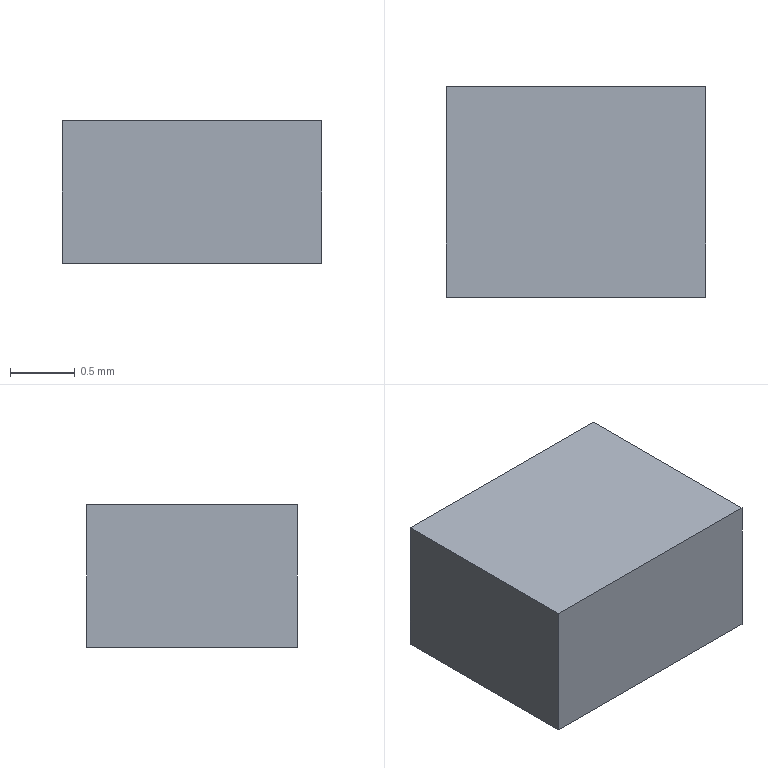Part | Creo | 1 solid | 6 faces | box 2 x 1.625 x 1.1 mm | volume 3.576 mm3 | plane 6
STEP:
#1=CARTESIAN_POINT('',(0.,0.,0.));
#2=DIRECTION('',(0.,0.,1.));
#3=DIRECTION('',(1.,0.,0.));
#4=AXIS2_PLACEMENT_3D('',#1,#2,#3);
#5=CARTESIAN_POINT('',(-1.,-0.8127,0.));
#6=VERTEX_POINT('',#5);
#7=CARTESIAN_POINT('',(1.,-0.8127,0.));
#8=VERTEX_POINT('',#7);
#9=CARTESIAN_POINT('',(-1.,-0.8127,0.));
#10=DIRECTION('',(1.,0.,0.));
#11=VECTOR('',#10,2.);
#12=LINE('',#9,#11);
#13=EDGE_CURVE('',#6,#8,#12,.T.);
#14=ORIENTED_EDGE('',*,*,#13,.T.);
#15=CARTESIAN_POINT('',(1.,0.8127,0.));
#16=VERTEX_POINT('',#15);
#17=CARTESIAN_POINT('',(1.,-0.8127,0.));
#18=DIRECTION('',(0.,1.,0.));
#19=VECTOR('',#18,1.625);
#20=LINE('',#17,#19);
#21=EDGE_CURVE('',#8,#16,#20,.T.);
#22=ORIENTED_EDGE('',*,*,#21,.T.);
#23=CARTESIAN_POINT('',(-1.,0.8127,0.));
#24=VERTEX_POINT('',#23);
#25=CARTESIAN_POINT('',(1.,0.8127,0.));
#26=DIRECTION('',(-1.,0.,0.));
#27=VECTOR('',#26,2.);
#28=LINE('',#25,#27);
#29=EDGE_CURVE('',#16,#24,#28,.T.);
#30=ORIENTED_EDGE('',*,*,#29,.T.);
#31=CARTESIAN_POINT('',(-1.,0.8127,0.));
#32=DIRECTION('',(0.,-1.,0.));
#33=VECTOR('',#32,1.625);
#34=LINE('',#31,#33);
#35=EDGE_CURVE('',#24,#6,#34,.T.);
#36=ORIENTED_EDGE('',*,*,#35,.T.);
#37=EDGE_LOOP('',(#14,#22,#30,#36));
#38=FACE_OUTER_BOUND('',#37,.F.);
#39=CARTESIAN_POINT('',(0.,0.,0.));
#40=DIRECTION('',(0.,0.,1.));
#41=DIRECTION('',(1.,0.,0.));
#42=AXIS2_PLACEMENT_3D('',#39,#40,#41);
#43=PLANE('',#42);
#44=ADVANCED_FACE('',(#38),#43,.F.);
#45=ORIENTED_EDGE('',*,*,#13,.F.);
#46=CARTESIAN_POINT('',(-1.,-0.8127,1.1));
#47=VERTEX_POINT('',#46);
#48=CARTESIAN_POINT('',(-1.,-0.8127,0.));
#49=DIRECTION('',(0.,0.,1.));
#50=VECTOR('',#49,1.1);
#51=LINE('',#48,#50);
#52=EDGE_CURVE('',#6,#47,#51,.T.);
#53=ORIENTED_EDGE('',*,*,#52,.T.);
#54=CARTESIAN_POINT('',(1.,-0.8127,1.1));
#55=VERTEX_POINT('',#54);
#56=CARTESIAN_POINT('',(-1.,-0.8127,1.1));
#57=DIRECTION('',(1.,0.,0.));
#58=VECTOR('',#57,2.);
#59=LINE('',#56,#58);
#60=EDGE_CURVE('',#47,#55,#59,.T.);
#61=ORIENTED_EDGE('',*,*,#60,.T.);
#62=CARTESIAN_POINT('',(1.,-0.8127,0.));
#63=DIRECTION('',(0.,0.,1.));
#64=VECTOR('',#63,1.1);
#65=LINE('',#62,#64);
#66=EDGE_CURVE('',#8,#55,#65,.T.);
#67=ORIENTED_EDGE('',*,*,#66,.F.);
#68=EDGE_LOOP('',(#45,#53,#61,#67));
#69=FACE_OUTER_BOUND('',#68,.F.);
#70=CARTESIAN_POINT('',(-1.,-0.8127,0.));
#71=DIRECTION('',(0.,-1.,0.));
#72=DIRECTION('',(1.,0.,0.));
#73=AXIS2_PLACEMENT_3D('',#70,#71,#72);
#74=PLANE('',#73);
#75=ADVANCED_FACE('',(#69),#74,.T.);
#76=ORIENTED_EDGE('',*,*,#35,.F.);
#77=CARTESIAN_POINT('',(-1.,0.8127,1.1));
#78=VERTEX_POINT('',#77);
#79=CARTESIAN_POINT('',(-1.,0.8127,0.));
#80=DIRECTION('',(0.,0.,1.));
#81=VECTOR('',#80,1.1);
#82=LINE('',#79,#81);
#83=EDGE_CURVE('',#24,#78,#82,.T.);
#84=ORIENTED_EDGE('',*,*,#83,.T.);
#85=CARTESIAN_POINT('',(-1.,0.8127,1.1));
#86=DIRECTION('',(0.,-1.,0.));
#87=VECTOR('',#86,1.625);
#88=LINE('',#85,#87);
#89=EDGE_CURVE('',#78,#47,#88,.T.);
#90=ORIENTED_EDGE('',*,*,#89,.T.);
#91=ORIENTED_EDGE('',*,*,#52,.F.);
#92=EDGE_LOOP('',(#76,#84,#90,#91));
#93=FACE_OUTER_BOUND('',#92,.F.);
#94=CARTESIAN_POINT('',(-1.,0.8127,0.));
#95=DIRECTION('',(-1.,0.,0.));
#96=DIRECTION('',(0.,-1.,0.));
#97=AXIS2_PLACEMENT_3D('',#94,#95,#96);
#98=PLANE('',#97);
#99=ADVANCED_FACE('',(#93),#98,.T.);
#100=ORIENTED_EDGE('',*,*,#29,.F.);
#101=CARTESIAN_POINT('',(1.,0.8127,1.1));
#102=VERTEX_POINT('',#101);
#103=CARTESIAN_POINT('',(1.,0.8127,0.));
#104=DIRECTION('',(0.,0.,1.));
#105=VECTOR('',#104,1.1);
#106=LINE('',#103,#105);
#107=EDGE_CURVE('',#16,#102,#106,.T.);
#108=ORIENTED_EDGE('',*,*,#107,.T.);
#109=CARTESIAN_POINT('',(1.,0.8127,1.1));
#110=DIRECTION('',(-1.,0.,0.));
#111=VECTOR('',#110,2.);
#112=LINE('',#109,#111);
#113=EDGE_CURVE('',#102,#78,#112,.T.);
#114=ORIENTED_EDGE('',*,*,#113,.T.);
#115=ORIENTED_EDGE('',*,*,#83,.F.);
#116=EDGE_LOOP('',(#100,#108,#114,#115));
#117=FACE_OUTER_BOUND('',#116,.F.);
#118=CARTESIAN_POINT('',(1.,0.8127,0.));
#119=DIRECTION('',(0.,1.,0.));
#120=DIRECTION('',(-1.,0.,0.));
#121=AXIS2_PLACEMENT_3D('',#118,#119,#120);
#122=PLANE('',#121);
#123=ADVANCED_FACE('',(#117),#122,.T.);
#124=ORIENTED_EDGE('',*,*,#21,.F.);
#125=ORIENTED_EDGE('',*,*,#66,.T.);
#126=CARTESIAN_POINT('',(1.,-0.8127,1.1));
#127=DIRECTION('',(0.,1.,0.));
#128=VECTOR('',#127,1.625);
#129=LINE('',#126,#128);
#130=EDGE_CURVE('',#55,#102,#129,.T.);
#131=ORIENTED_EDGE('',*,*,#130,.T.);
#132=ORIENTED_EDGE('',*,*,#107,.F.);
#133=EDGE_LOOP('',(#124,#125,#131,#132));
#134=FACE_OUTER_BOUND('',#133,.F.);
#135=CARTESIAN_POINT('',(1.,-0.8127,0.));
#136=DIRECTION('',(1.,0.,0.));
#137=DIRECTION('',(0.,1.,0.));
#138=AXIS2_PLACEMENT_3D('',#135,#136,#137);
#139=PLANE('',#138);
#140=ADVANCED_FACE('',(#134),#139,.T.);
#141=ORIENTED_EDGE('',*,*,#60,.F.);
#142=ORIENTED_EDGE('',*,*,#89,.F.);
#143=ORIENTED_EDGE('',*,*,#113,.F.);
#144=ORIENTED_EDGE('',*,*,#130,.F.);
#145=EDGE_LOOP('',(#141,#142,#143,#144));
#146=FACE_OUTER_BOUND('',#145,.F.);
#147=CARTESIAN_POINT('',(0.,0.,1.1));
#148=DIRECTION('',(0.,0.,1.));
#149=DIRECTION('',(1.,0.,0.));
#150=AXIS2_PLACEMENT_3D('',#147,#148,#149);
#151=PLANE('',#150);
#152=ADVANCED_FACE('',(#146),#151,.T.);
#153=CLOSED_SHELL('',(#44,#75,#99,#123,#140,#152));
#154=MANIFOLD_SOLID_BREP('',#153);
#155=(LENGTH_UNIT()NAMED_UNIT(*)SI_UNIT(.MILLI.,.METRE.));
#156=UNCERTAINTY_MEASURE_WITH_UNIT(LENGTH_MEASURE(0.0002802),#155,'','');
#157=(NAMED_UNIT(*)PLANE_ANGLE_UNIT()SI_UNIT($,.RADIAN.));
#158=PLANE_ANGLE_MEASURE_WITH_UNIT(PLANE_ANGLE_MEASURE(0.01745),#157);
#159=(CONVERSION_BASED_UNIT('DEGREE',#158)NAMED_UNIT(*)PLANE_ANGLE_UNIT());
#160=(NAMED_UNIT(*)SI_UNIT($,.STERADIAN.)SOLID_ANGLE_UNIT());
#161=(GEOMETRIC_REPRESENTATION_CONTEXT(3)GLOBAL_UNCERTAINTY_ASSIGNED_CONTEXT((#156))GLOBAL_UNIT_ASSIGNED_CONTEXT((#155,#159,#160))REPRESENTATION_CONTEXT('',''));
#162=ADVANCED_BREP_SHAPE_REPRESENTATION('',(#4,#154),#161);